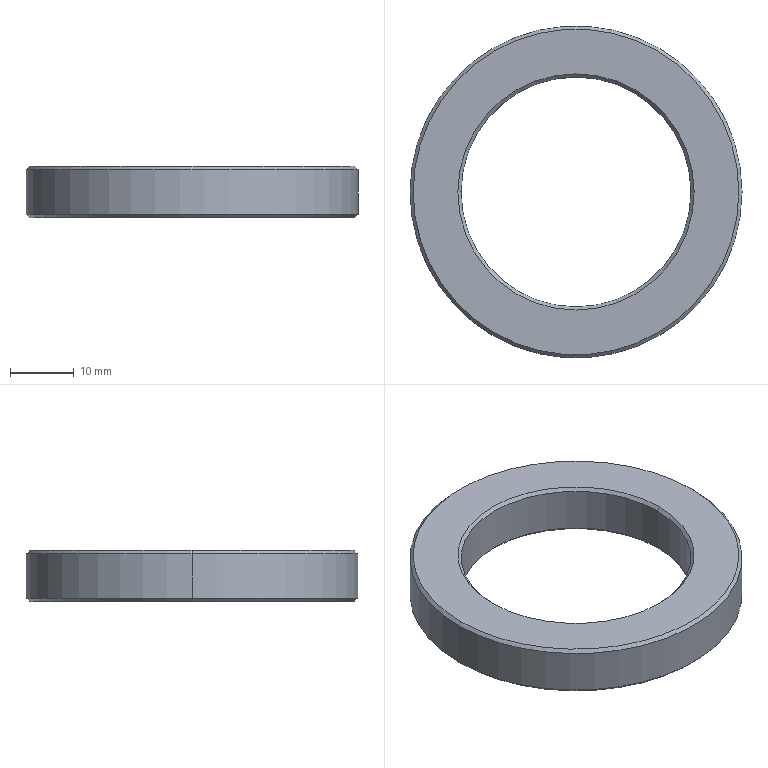Part | SolidWorks | features Chamfer 1, Extrusion 1 | 1 solid | 14 faces | box 52 x 52 x 8 mm | volume 8778 mm3 | cone 8 | cylinder 4 | plane 2 | commonest cylinder face diameters 36 x2 52 x2
STEP:
#1=CARTESIAN_POINT('',(-18.,0.,7.5));
#2=VERTEX_POINT('',#1);
#3=CARTESIAN_POINT('',(18.,0.,7.5));
#4=VERTEX_POINT('',#3);
#5=CARTESIAN_POINT('',(0.,0.,7.5));
#6=DIRECTION('',(0.,0.,1.));
#7=DIRECTION('',(1.,0.,0.));
#8=AXIS2_PLACEMENT_3D('',#5,#6,#7);
#9=CIRCLE('',#8,18.);
#10=EDGE_CURVE('',#2,#4,#9,.T.);
#11=ORIENTED_EDGE('',*,*,#10,.F.);
#12=CARTESIAN_POINT('',(-18.5,0.,8.));
#13=VERTEX_POINT('',#12);
#14=CARTESIAN_POINT('',(-18.,0.,7.5));
#15=DIRECTION('',(-0.7071,0.,0.7071));
#16=VECTOR('',#15,1000.);
#17=LINE('',#14,#16);
#18=EDGE_CURVE('',#2,#13,#17,.T.);
#19=ORIENTED_EDGE('',*,*,#18,.T.);
#20=CARTESIAN_POINT('',(18.5,0.,8.));
#21=VERTEX_POINT('',#20);
#22=CARTESIAN_POINT('',(0.,0.,8.));
#23=DIRECTION('',(0.,0.,-1.));
#24=DIRECTION('',(1.,0.,0.));
#25=AXIS2_PLACEMENT_3D('',#22,#23,#24);
#26=CIRCLE('',#25,18.5);
#27=EDGE_CURVE('',#21,#13,#26,.T.);
#28=ORIENTED_EDGE('',*,*,#27,.F.);
#29=CARTESIAN_POINT('',(18.,0.,7.5));
#30=DIRECTION('',(0.7071,0.,0.7071));
#31=VECTOR('',#30,1000.);
#32=LINE('',#29,#31);
#33=EDGE_CURVE('',#4,#21,#32,.T.);
#34=ORIENTED_EDGE('',*,*,#33,.F.);
#35=EDGE_LOOP('',(#11,#19,#28,#34));
#36=FACE_OUTER_BOUND('',#35,.T.);
#37=CARTESIAN_POINT('',(0.,0.,7.5));
#38=DIRECTION('',(0.,0.,1.));
#39=DIRECTION('',(1.,0.,0.));
#40=AXIS2_PLACEMENT_3D('',#37,#38,#39);
#41=CONICAL_SURFACE('',#40,18.,0.7854);
#42=ADVANCED_FACE('',(#36),#41,.F.);
#43=CARTESIAN_POINT('',(18.,0.,0.5));
#44=VERTEX_POINT('',#43);
#45=CARTESIAN_POINT('',(-18.,0.,0.5));
#46=VERTEX_POINT('',#45);
#47=CARTESIAN_POINT('',(0.,0.,0.5));
#48=DIRECTION('',(0.,0.,-1.));
#49=DIRECTION('',(1.,0.,0.));
#50=AXIS2_PLACEMENT_3D('',#47,#48,#49);
#51=CIRCLE('',#50,18.);
#52=EDGE_CURVE('',#44,#46,#51,.T.);
#53=ORIENTED_EDGE('',*,*,#52,.F.);
#54=CARTESIAN_POINT('',(18.5,0.,0.));
#55=VERTEX_POINT('',#54);
#56=CARTESIAN_POINT('',(18.5,0.,0.));
#57=DIRECTION('',(0.7071,0.,-0.7071));
#58=VECTOR('',#57,1000.);
#59=LINE('',#56,#58);
#60=EDGE_CURVE('',#44,#55,#59,.T.);
#61=ORIENTED_EDGE('',*,*,#60,.T.);
#62=CARTESIAN_POINT('',(-18.5,0.,0.));
#63=VERTEX_POINT('',#62);
#64=CARTESIAN_POINT('',(0.,0.,0.));
#65=DIRECTION('',(0.,0.,1.));
#66=DIRECTION('',(1.,0.,0.));
#67=AXIS2_PLACEMENT_3D('',#64,#65,#66);
#68=CIRCLE('',#67,18.5);
#69=EDGE_CURVE('',#63,#55,#68,.T.);
#70=ORIENTED_EDGE('',*,*,#69,.F.);
#71=CARTESIAN_POINT('',(-18.5,0.,0.));
#72=DIRECTION('',(-0.7071,0.,-0.7071));
#73=VECTOR('',#72,1000.);
#74=LINE('',#71,#73);
#75=EDGE_CURVE('',#46,#63,#74,.T.);
#76=ORIENTED_EDGE('',*,*,#75,.F.);
#77=EDGE_LOOP('',(#53,#61,#70,#76));
#78=FACE_OUTER_BOUND('',#77,.T.);
#79=CARTESIAN_POINT('',(0.,0.,0.));
#80=DIRECTION('',(0.,0.,-1.));
#81=DIRECTION('',(-1.,0.,0.));
#82=AXIS2_PLACEMENT_3D('',#79,#80,#81);
#83=CONICAL_SURFACE('',#82,18.5,0.7854);
#84=ADVANCED_FACE('',(#78),#83,.F.);
#85=CARTESIAN_POINT('',(-25.5,0.,0.));
#86=VERTEX_POINT('',#85);
#87=CARTESIAN_POINT('',(25.5,0.,0.));
#88=VERTEX_POINT('',#87);
#89=CARTESIAN_POINT('',(0.,0.,0.));
#90=DIRECTION('',(0.,0.,-1.));
#91=DIRECTION('',(1.,0.,0.));
#92=AXIS2_PLACEMENT_3D('',#89,#90,#91);
#93=CIRCLE('',#92,25.5);
#94=EDGE_CURVE('',#86,#88,#93,.T.);
#95=ORIENTED_EDGE('',*,*,#94,.F.);
#96=CARTESIAN_POINT('',(-26.,0.,0.5));
#97=VERTEX_POINT('',#96);
#98=CARTESIAN_POINT('',(-26.,0.,0.5));
#99=DIRECTION('',(-0.7071,0.,0.7071));
#100=VECTOR('',#99,1000.);
#101=LINE('',#98,#100);
#102=EDGE_CURVE('',#86,#97,#101,.T.);
#103=ORIENTED_EDGE('',*,*,#102,.T.);
#104=CARTESIAN_POINT('',(26.,0.,0.5));
#105=VERTEX_POINT('',#104);
#106=CARTESIAN_POINT('',(0.,0.,0.5));
#107=DIRECTION('',(0.,0.,1.));
#108=DIRECTION('',(1.,0.,0.));
#109=AXIS2_PLACEMENT_3D('',#106,#107,#108);
#110=CIRCLE('',#109,26.);
#111=EDGE_CURVE('',#105,#97,#110,.T.);
#112=ORIENTED_EDGE('',*,*,#111,.F.);
#113=CARTESIAN_POINT('',(26.,0.,0.5));
#114=DIRECTION('',(0.7071,0.,0.7071));
#115=VECTOR('',#114,1000.);
#116=LINE('',#113,#115);
#117=EDGE_CURVE('',#88,#105,#116,.T.);
#118=ORIENTED_EDGE('',*,*,#117,.F.);
#119=EDGE_LOOP('',(#95,#103,#112,#118));
#120=FACE_OUTER_BOUND('',#119,.T.);
#121=CARTESIAN_POINT('',(0.,0.,0.5));
#122=DIRECTION('',(0.,0.,1.));
#123=DIRECTION('',(1.,0.,0.));
#124=AXIS2_PLACEMENT_3D('',#121,#122,#123);
#125=CONICAL_SURFACE('',#124,26.,0.7854);
#126=ADVANCED_FACE('',(#120),#125,.T.);
#127=CARTESIAN_POINT('',(25.5,0.,8.));
#128=VERTEX_POINT('',#127);
#129=CARTESIAN_POINT('',(-25.5,0.,8.));
#130=VERTEX_POINT('',#129);
#131=CARTESIAN_POINT('',(0.,0.,8.));
#132=DIRECTION('',(0.,0.,1.));
#133=DIRECTION('',(1.,0.,0.));
#134=AXIS2_PLACEMENT_3D('',#131,#132,#133);
#135=CIRCLE('',#134,25.5);
#136=EDGE_CURVE('',#128,#130,#135,.T.);
#137=ORIENTED_EDGE('',*,*,#136,.F.);
#138=CARTESIAN_POINT('',(26.,0.,7.5));
#139=VERTEX_POINT('',#138);
#140=CARTESIAN_POINT('',(25.5,0.,8.));
#141=DIRECTION('',(0.7071,0.,-0.7071));
#142=VECTOR('',#141,1000.);
#143=LINE('',#140,#142);
#144=EDGE_CURVE('',#128,#139,#143,.T.);
#145=ORIENTED_EDGE('',*,*,#144,.T.);
#146=CARTESIAN_POINT('',(-26.,0.,7.5));
#147=VERTEX_POINT('',#146);
#148=CARTESIAN_POINT('',(0.,0.,7.5));
#149=DIRECTION('',(0.,0.,-1.));
#150=DIRECTION('',(1.,0.,0.));
#151=AXIS2_PLACEMENT_3D('',#148,#149,#150);
#152=CIRCLE('',#151,26.);
#153=EDGE_CURVE('',#147,#139,#152,.T.);
#154=ORIENTED_EDGE('',*,*,#153,.F.);
#155=CARTESIAN_POINT('',(-25.5,0.,8.));
#156=DIRECTION('',(-0.7071,0.,-0.7071));
#157=VECTOR('',#156,1000.);
#158=LINE('',#155,#157);
#159=EDGE_CURVE('',#130,#147,#158,.T.);
#160=ORIENTED_EDGE('',*,*,#159,.F.);
#161=EDGE_LOOP('',(#137,#145,#154,#160));
#162=FACE_OUTER_BOUND('',#161,.T.);
#163=CARTESIAN_POINT('',(0.,0.,8.));
#164=DIRECTION('',(0.,0.,-1.));
#165=DIRECTION('',(-1.,0.,0.));
#166=AXIS2_PLACEMENT_3D('',#163,#164,#165);
#167=CONICAL_SURFACE('',#166,25.5,0.7854);
#168=ADVANCED_FACE('',(#162),#167,.T.);
#169=ORIENTED_EDGE('',*,*,#10,.T.);
#170=CARTESIAN_POINT('',(18.,0.,8.));
#171=DIRECTION('',(0.,0.,-1.));
#172=VECTOR('',#171,1000.);
#173=LINE('',#170,#172);
#174=EDGE_CURVE('',#4,#44,#173,.T.);
#175=ORIENTED_EDGE('',*,*,#174,.T.);
#176=ORIENTED_EDGE('',*,*,#52,.T.);
#177=CARTESIAN_POINT('',(-18.,0.,8.));
#178=DIRECTION('',(0.,0.,-1.));
#179=VECTOR('',#178,1000.);
#180=LINE('',#177,#179);
#181=EDGE_CURVE('',#2,#46,#180,.T.);
#182=ORIENTED_EDGE('',*,*,#181,.F.);
#183=EDGE_LOOP('',(#169,#175,#176,#182));
#184=FACE_OUTER_BOUND('',#183,.T.);
#185=CARTESIAN_POINT('',(0.,0.,8.));
#186=DIRECTION('',(0.,0.,-1.));
#187=DIRECTION('',(-1.,0.,0.));
#188=AXIS2_PLACEMENT_3D('',#185,#186,#187);
#189=CYLINDRICAL_SURFACE('',#188,18.);
#190=ADVANCED_FACE('',(#184),#189,.F.);
#191=ORIENTED_EDGE('',*,*,#153,.T.);
#192=CARTESIAN_POINT('',(26.,0.,8.));
#193=DIRECTION('',(0.,0.,-1.));
#194=VECTOR('',#193,1000.);
#195=LINE('',#192,#194);
#196=EDGE_CURVE('',#139,#105,#195,.T.);
#197=ORIENTED_EDGE('',*,*,#196,.T.);
#198=ORIENTED_EDGE('',*,*,#111,.T.);
#199=CARTESIAN_POINT('',(-26.,0.,8.));
#200=DIRECTION('',(0.,0.,-1.));
#201=VECTOR('',#200,1000.);
#202=LINE('',#199,#201);
#203=EDGE_CURVE('',#147,#97,#202,.T.);
#204=ORIENTED_EDGE('',*,*,#203,.F.);
#205=EDGE_LOOP('',(#191,#197,#198,#204));
#206=FACE_OUTER_BOUND('',#205,.T.);
#207=CARTESIAN_POINT('',(0.,0.,8.));
#208=DIRECTION('',(0.,0.,-1.));
#209=DIRECTION('',(-1.,0.,0.));
#210=AXIS2_PLACEMENT_3D('',#207,#208,#209);
#211=CYLINDRICAL_SURFACE('',#210,26.);
#212=ADVANCED_FACE('',(#206),#211,.T.);
#213=CARTESIAN_POINT('',(0.,0.,8.));
#214=DIRECTION('',(0.,0.,1.));
#215=DIRECTION('',(1.,0.,0.));
#216=AXIS2_PLACEMENT_3D('',#213,#214,#215);
#217=CIRCLE('',#216,25.5);
#218=EDGE_CURVE('',#130,#128,#217,.T.);
#219=ORIENTED_EDGE('',*,*,#218,.T.);
#220=ORIENTED_EDGE('',*,*,#136,.T.);
#221=EDGE_LOOP('',(#219,#220));
#222=FACE_OUTER_BOUND('',#221,.T.);
#223=ORIENTED_EDGE('',*,*,#27,.T.);
#224=CARTESIAN_POINT('',(0.,0.,8.));
#225=DIRECTION('',(0.,0.,-1.));
#226=DIRECTION('',(1.,0.,0.));
#227=AXIS2_PLACEMENT_3D('',#224,#225,#226);
#228=CIRCLE('',#227,18.5);
#229=EDGE_CURVE('',#13,#21,#228,.T.);
#230=ORIENTED_EDGE('',*,*,#229,.T.);
#231=EDGE_LOOP('',(#223,#230));
#232=FACE_BOUND('',#231,.T.);
#233=CARTESIAN_POINT('',(0.,0.,8.));
#234=DIRECTION('',(0.,0.,1.));
#235=DIRECTION('',(1.,0.,0.));
#236=AXIS2_PLACEMENT_3D('',#233,#234,#235);
#237=PLANE('',#236);
#238=ADVANCED_FACE('',(#222,#232),#237,.T.);
#239=CARTESIAN_POINT('',(0.,0.,0.));
#240=DIRECTION('',(0.,0.,-1.));
#241=DIRECTION('',(1.,0.,0.));
#242=AXIS2_PLACEMENT_3D('',#239,#240,#241);
#243=CIRCLE('',#242,25.5);
#244=EDGE_CURVE('',#88,#86,#243,.T.);
#245=ORIENTED_EDGE('',*,*,#244,.T.);
#246=ORIENTED_EDGE('',*,*,#94,.T.);
#247=EDGE_LOOP('',(#245,#246));
#248=FACE_OUTER_BOUND('',#247,.T.);
#249=ORIENTED_EDGE('',*,*,#69,.T.);
#250=CARTESIAN_POINT('',(0.,0.,0.));
#251=DIRECTION('',(0.,0.,1.));
#252=DIRECTION('',(1.,0.,0.));
#253=AXIS2_PLACEMENT_3D('',#250,#251,#252);
#254=CIRCLE('',#253,18.5);
#255=EDGE_CURVE('',#55,#63,#254,.T.);
#256=ORIENTED_EDGE('',*,*,#255,.T.);
#257=EDGE_LOOP('',(#249,#256));
#258=FACE_BOUND('',#257,.T.);
#259=CARTESIAN_POINT('',(0.,0.,0.));
#260=DIRECTION('',(0.,0.,1.));
#261=DIRECTION('',(1.,0.,0.));
#262=AXIS2_PLACEMENT_3D('',#259,#260,#261);
#263=PLANE('',#262);
#264=ADVANCED_FACE('',(#248,#258),#263,.F.);
#265=ORIENTED_EDGE('',*,*,#196,.F.);
#266=CARTESIAN_POINT('',(0.,0.,7.5));
#267=DIRECTION('',(0.,0.,-1.));
#268=DIRECTION('',(1.,0.,0.));
#269=AXIS2_PLACEMENT_3D('',#266,#267,#268);
#270=CIRCLE('',#269,26.);
#271=EDGE_CURVE('',#139,#147,#270,.T.);
#272=ORIENTED_EDGE('',*,*,#271,.T.);
#273=ORIENTED_EDGE('',*,*,#203,.T.);
#274=CARTESIAN_POINT('',(0.,0.,0.5));
#275=DIRECTION('',(0.,0.,1.));
#276=DIRECTION('',(1.,0.,0.));
#277=AXIS2_PLACEMENT_3D('',#274,#275,#276);
#278=CIRCLE('',#277,26.);
#279=EDGE_CURVE('',#97,#105,#278,.T.);
#280=ORIENTED_EDGE('',*,*,#279,.T.);
#281=EDGE_LOOP('',(#265,#272,#273,#280));
#282=FACE_OUTER_BOUND('',#281,.T.);
#283=CARTESIAN_POINT('',(0.,0.,8.));
#284=DIRECTION('',(0.,0.,-1.));
#285=DIRECTION('',(-1.,0.,0.));
#286=AXIS2_PLACEMENT_3D('',#283,#284,#285);
#287=CYLINDRICAL_SURFACE('',#286,26.);
#288=ADVANCED_FACE('',(#282),#287,.T.);
#289=ORIENTED_EDGE('',*,*,#174,.F.);
#290=CARTESIAN_POINT('',(0.,0.,7.5));
#291=DIRECTION('',(0.,0.,1.));
#292=DIRECTION('',(1.,0.,0.));
#293=AXIS2_PLACEMENT_3D('',#290,#291,#292);
#294=CIRCLE('',#293,18.);
#295=EDGE_CURVE('',#4,#2,#294,.T.);
#296=ORIENTED_EDGE('',*,*,#295,.T.);
#297=ORIENTED_EDGE('',*,*,#181,.T.);
#298=CARTESIAN_POINT('',(0.,0.,0.5));
#299=DIRECTION('',(0.,0.,-1.));
#300=DIRECTION('',(1.,0.,0.));
#301=AXIS2_PLACEMENT_3D('',#298,#299,#300);
#302=CIRCLE('',#301,18.);
#303=EDGE_CURVE('',#46,#44,#302,.T.);
#304=ORIENTED_EDGE('',*,*,#303,.T.);
#305=EDGE_LOOP('',(#289,#296,#297,#304));
#306=FACE_OUTER_BOUND('',#305,.T.);
#307=CARTESIAN_POINT('',(0.,0.,8.));
#308=DIRECTION('',(0.,0.,-1.));
#309=DIRECTION('',(-1.,0.,0.));
#310=AXIS2_PLACEMENT_3D('',#307,#308,#309);
#311=CYLINDRICAL_SURFACE('',#310,18.);
#312=ADVANCED_FACE('',(#306),#311,.F.);
#313=ORIENTED_EDGE('',*,*,#144,.F.);
#314=ORIENTED_EDGE('',*,*,#218,.F.);
#315=ORIENTED_EDGE('',*,*,#159,.T.);
#316=ORIENTED_EDGE('',*,*,#271,.F.);
#317=EDGE_LOOP('',(#313,#314,#315,#316));
#318=FACE_OUTER_BOUND('',#317,.T.);
#319=CARTESIAN_POINT('',(0.,0.,8.));
#320=DIRECTION('',(0.,0.,-1.));
#321=DIRECTION('',(-1.,0.,0.));
#322=AXIS2_PLACEMENT_3D('',#319,#320,#321);
#323=CONICAL_SURFACE('',#322,25.5,0.7854);
#324=ADVANCED_FACE('',(#318),#323,.T.);
#325=ORIENTED_EDGE('',*,*,#102,.F.);
#326=ORIENTED_EDGE('',*,*,#244,.F.);
#327=ORIENTED_EDGE('',*,*,#117,.T.);
#328=ORIENTED_EDGE('',*,*,#279,.F.);
#329=EDGE_LOOP('',(#325,#326,#327,#328));
#330=FACE_OUTER_BOUND('',#329,.T.);
#331=CARTESIAN_POINT('',(0.,0.,0.5));
#332=DIRECTION('',(0.,0.,1.));
#333=DIRECTION('',(1.,0.,0.));
#334=AXIS2_PLACEMENT_3D('',#331,#332,#333);
#335=CONICAL_SURFACE('',#334,26.,0.7854);
#336=ADVANCED_FACE('',(#330),#335,.T.);
#337=ORIENTED_EDGE('',*,*,#60,.F.);
#338=ORIENTED_EDGE('',*,*,#303,.F.);
#339=ORIENTED_EDGE('',*,*,#75,.T.);
#340=ORIENTED_EDGE('',*,*,#255,.F.);
#341=EDGE_LOOP('',(#337,#338,#339,#340));
#342=FACE_OUTER_BOUND('',#341,.T.);
#343=CARTESIAN_POINT('',(0.,0.,0.));
#344=DIRECTION('',(0.,0.,-1.));
#345=DIRECTION('',(-1.,0.,0.));
#346=AXIS2_PLACEMENT_3D('',#343,#344,#345);
#347=CONICAL_SURFACE('',#346,18.5,0.7854);
#348=ADVANCED_FACE('',(#342),#347,.F.);
#349=ORIENTED_EDGE('',*,*,#18,.F.);
#350=ORIENTED_EDGE('',*,*,#295,.F.);
#351=ORIENTED_EDGE('',*,*,#33,.T.);
#352=ORIENTED_EDGE('',*,*,#229,.F.);
#353=EDGE_LOOP('',(#349,#350,#351,#352));
#354=FACE_OUTER_BOUND('',#353,.T.);
#355=CARTESIAN_POINT('',(0.,0.,7.5));
#356=DIRECTION('',(0.,0.,1.));
#357=DIRECTION('',(1.,0.,0.));
#358=AXIS2_PLACEMENT_3D('',#355,#356,#357);
#359=CONICAL_SURFACE('',#358,18.,0.7854);
#360=ADVANCED_FACE('',(#354),#359,.F.);
#361=CLOSED_SHELL('',(#42,#84,#126,#168,#190,#212,#238,#264,#288,#312,#324,#336,#348,#360));
#362=MANIFOLD_SOLID_BREP('',#361);
#363=CARTESIAN_POINT('',(0.,0.,0.));
#364=DIRECTION('',(0.,0.,1.));
#365=DIRECTION('',(1.,0.,0.));
#366=AXIS2_PLACEMENT_3D('',#363,#364,#365);
#367=(LENGTH_UNIT()NAMED_UNIT(*)SI_UNIT(.MILLI.,.METRE.));
#368=UNCERTAINTY_MEASURE_WITH_UNIT(LENGTH_MEASURE(0.00001),#367,'','');
#369=(NAMED_UNIT(*)PLANE_ANGLE_UNIT()SI_UNIT($,.RADIAN.));
#370=(NAMED_UNIT(*)SI_UNIT($,.STERADIAN.)SOLID_ANGLE_UNIT());
#371=(GEOMETRIC_REPRESENTATION_CONTEXT(3)GLOBAL_UNCERTAINTY_ASSIGNED_CONTEXT((#368))GLOBAL_UNIT_ASSIGNED_CONTEXT((#367,#369,#370))REPRESENTATION_CONTEXT('',''));
#372=ADVANCED_BREP_SHAPE_REPRESENTATION('',(#362,#366),#371);